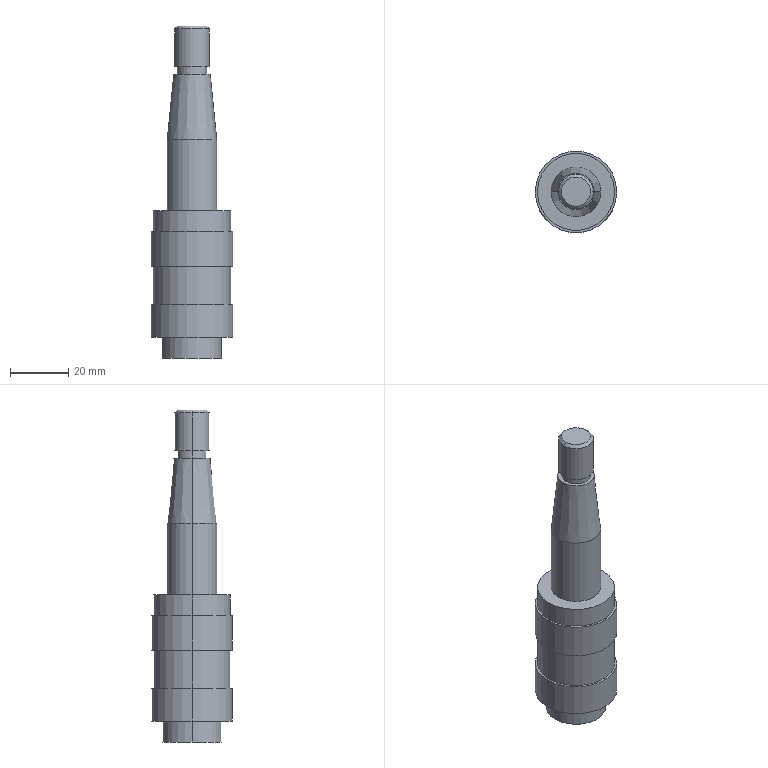Part | SolidWorks | features BaseBody 1 | 1 solid | 29 faces | box 28 x 28 x 114 mm | volume 38900 mm3 | cylinder 16 | plane 9 | cone 4 | commonest cylinder face diameters 26.5 x4 28 x4 10 x2 12 x2 17 x2 20.275 x2
STEP:
#1=CARTESIAN_POINT('',(0.5987,-67.08,58.));
#2=VERTEX_POINT('',#1);
#3=CARTESIAN_POINT('',(-16.401,-67.08,58.));
#4=VERTEX_POINT('',#3);
#5=CARTESIAN_POINT('',(-7.901,-67.08,58.));
#6=DIRECTION('',(0.,0.,1.));
#7=DIRECTION('',(1.,0.,0.));
#8=AXIS2_PLACEMENT_3D('',#5,#6,#7);
#9=CIRCLE('',#8,8.5);
#10=EDGE_CURVE('',#2,#4,#9,.T.);
#11=ORIENTED_EDGE('',*,*,#10,.T.);
#12=CARTESIAN_POINT('',(-16.401,-67.08,82.499));
#13=VERTEX_POINT('',#12);
#14=CARTESIAN_POINT('',(-16.401,-67.08,58.));
#15=DIRECTION('',(0.,0.,1.));
#16=VECTOR('',#15,1000.);
#17=LINE('',#14,#16);
#18=EDGE_CURVE('',#4,#13,#17,.T.);
#19=ORIENTED_EDGE('',*,*,#18,.T.);
#20=CARTESIAN_POINT('',(0.5987,-67.08,82.499));
#21=VERTEX_POINT('',#20);
#22=CARTESIAN_POINT('',(-7.901,-67.08,82.499));
#23=DIRECTION('',(0.,0.,-1.));
#24=DIRECTION('',(1.,0.,0.));
#25=AXIS2_PLACEMENT_3D('',#22,#23,#24);
#26=CIRCLE('',#25,8.5);
#27=EDGE_CURVE('',#13,#21,#26,.T.);
#28=ORIENTED_EDGE('',*,*,#27,.T.);
#29=CARTESIAN_POINT('',(0.5987,-67.08,58.));
#30=DIRECTION('',(0.,0.,1.));
#31=VECTOR('',#30,1000.);
#32=LINE('',#29,#31);
#33=EDGE_CURVE('',#2,#21,#32,.T.);
#34=ORIENTED_EDGE('',*,*,#33,.F.);
#35=EDGE_LOOP('',(#11,#19,#28,#34));
#36=FACE_OUTER_BOUND('',#35,.T.);
#37=CARTESIAN_POINT('',(-7.901,-67.08,58.));
#38=DIRECTION('',(0.,0.,1.));
#39=DIRECTION('',(1.,0.,0.));
#40=AXIS2_PLACEMENT_3D('',#37,#38,#39);
#41=CYLINDRICAL_SURFACE('',#40,8.5);
#42=ADVANCED_FACE('',(#36),#41,.T.);
#43=CARTESIAN_POINT('',(-14.151,-67.08,105.));
#44=VERTEX_POINT('',#43);
#45=CARTESIAN_POINT('',(-1.651,-67.08,105.));
#46=VERTEX_POINT('',#45);
#47=CARTESIAN_POINT('',(-7.901,-67.08,105.));
#48=DIRECTION('',(0.,0.,-1.));
#49=DIRECTION('',(-1.,0.,0.));
#50=AXIS2_PLACEMENT_3D('',#47,#48,#49);
#51=CIRCLE('',#50,6.25);
#52=EDGE_CURVE('',#44,#46,#51,.T.);
#53=ORIENTED_EDGE('',*,*,#52,.T.);
#54=CARTESIAN_POINT('',(0.5987,-67.08,82.499));
#55=DIRECTION('',(0.09949,0.,-0.995));
#56=VECTOR('',#55,1000.);
#57=LINE('',#54,#56);
#58=EDGE_CURVE('',#46,#21,#57,.T.);
#59=ORIENTED_EDGE('',*,*,#58,.T.);
#60=ORIENTED_EDGE('',*,*,#27,.F.);
#61=CARTESIAN_POINT('',(-16.401,-67.08,82.499));
#62=DIRECTION('',(-0.09949,0.,-0.995));
#63=VECTOR('',#62,1000.);
#64=LINE('',#61,#63);
#65=EDGE_CURVE('',#44,#13,#64,.T.);
#66=ORIENTED_EDGE('',*,*,#65,.F.);
#67=EDGE_LOOP('',(#53,#59,#60,#66));
#68=FACE_OUTER_BOUND('',#67,.T.);
#69=CARTESIAN_POINT('',(-7.901,-67.08,82.499));
#70=DIRECTION('',(0.,0.,-1.));
#71=DIRECTION('',(-1.,0.,0.));
#72=AXIS2_PLACEMENT_3D('',#69,#70,#71);
#73=CONICAL_SURFACE('',#72,8.5,0.09966);
#74=ADVANCED_FACE('',(#68),#73,.T.);
#75=CARTESIAN_POINT('',(5.349,-67.08,51.));
#76=VERTEX_POINT('',#75);
#77=CARTESIAN_POINT('',(-21.151,-67.08,51.));
#78=VERTEX_POINT('',#77);
#79=CARTESIAN_POINT('',(-7.901,-67.08,51.));
#80=DIRECTION('',(0.,0.,1.));
#81=DIRECTION('',(1.,0.,0.));
#82=AXIS2_PLACEMENT_3D('',#79,#80,#81);
#83=CIRCLE('',#82,13.25);
#84=EDGE_CURVE('',#76,#78,#83,.T.);
#85=ORIENTED_EDGE('',*,*,#84,.T.);
#86=CARTESIAN_POINT('',(-21.151,-67.08,58.));
#87=VERTEX_POINT('',#86);
#88=CARTESIAN_POINT('',(-21.151,-67.08,51.));
#89=DIRECTION('',(0.,0.,1.));
#90=VECTOR('',#89,1000.);
#91=LINE('',#88,#90);
#92=EDGE_CURVE('',#78,#87,#91,.T.);
#93=ORIENTED_EDGE('',*,*,#92,.T.);
#94=CARTESIAN_POINT('',(5.349,-67.08,58.));
#95=VERTEX_POINT('',#94);
#96=CARTESIAN_POINT('',(-7.901,-67.08,58.));
#97=DIRECTION('',(0.,0.,1.));
#98=DIRECTION('',(1.,0.,0.));
#99=AXIS2_PLACEMENT_3D('',#96,#97,#98);
#100=CIRCLE('',#99,13.25);
#101=EDGE_CURVE('',#95,#87,#100,.T.);
#102=ORIENTED_EDGE('',*,*,#101,.F.);
#103=CARTESIAN_POINT('',(5.349,-67.08,51.));
#104=DIRECTION('',(0.,0.,1.));
#105=VECTOR('',#104,1000.);
#106=LINE('',#103,#105);
#107=EDGE_CURVE('',#76,#95,#106,.T.);
#108=ORIENTED_EDGE('',*,*,#107,.F.);
#109=EDGE_LOOP('',(#85,#93,#102,#108));
#110=FACE_OUTER_BOUND('',#109,.T.);
#111=CARTESIAN_POINT('',(-7.901,-67.08,51.));
#112=DIRECTION('',(0.,0.,1.));
#113=DIRECTION('',(1.,0.,0.));
#114=AXIS2_PLACEMENT_3D('',#111,#112,#113);
#115=CYLINDRICAL_SURFACE('',#114,13.25);
#116=ADVANCED_FACE('',(#110),#115,.T.);
#117=CARTESIAN_POINT('',(-12.901,-67.08,105.));
#118=VERTEX_POINT('',#117);
#119=CARTESIAN_POINT('',(-2.901,-67.08,105.));
#120=VERTEX_POINT('',#119);
#121=CARTESIAN_POINT('',(-7.901,-67.08,105.));
#122=DIRECTION('',(0.,0.,-1.));
#123=DIRECTION('',(1.,0.,0.));
#124=AXIS2_PLACEMENT_3D('',#121,#122,#123);
#125=CIRCLE('',#124,5.);
#126=EDGE_CURVE('',#118,#120,#125,.T.);
#127=ORIENTED_EDGE('',*,*,#126,.F.);
#128=CARTESIAN_POINT('',(-12.901,-67.08,107.5));
#129=VERTEX_POINT('',#128);
#130=CARTESIAN_POINT('',(-12.901,-67.08,105.));
#131=DIRECTION('',(0.,0.,1.));
#132=VECTOR('',#131,1000.);
#133=LINE('',#130,#132);
#134=EDGE_CURVE('',#118,#129,#133,.T.);
#135=ORIENTED_EDGE('',*,*,#134,.T.);
#136=CARTESIAN_POINT('',(-2.901,-67.08,107.5));
#137=VERTEX_POINT('',#136);
#138=CARTESIAN_POINT('',(-7.901,-67.08,107.5));
#139=DIRECTION('',(0.,0.,-1.));
#140=DIRECTION('',(1.,0.,0.));
#141=AXIS2_PLACEMENT_3D('',#138,#139,#140);
#142=CIRCLE('',#141,5.);
#143=EDGE_CURVE('',#129,#137,#142,.T.);
#144=ORIENTED_EDGE('',*,*,#143,.T.);
#145=CARTESIAN_POINT('',(-2.901,-67.08,105.));
#146=DIRECTION('',(0.,0.,1.));
#147=VECTOR('',#146,1000.);
#148=LINE('',#145,#147);
#149=EDGE_CURVE('',#120,#137,#148,.T.);
#150=ORIENTED_EDGE('',*,*,#149,.F.);
#151=EDGE_LOOP('',(#127,#135,#144,#150));
#152=FACE_OUTER_BOUND('',#151,.T.);
#153=CARTESIAN_POINT('',(-7.901,-67.08,105.));
#154=DIRECTION('',(0.,0.,1.));
#155=DIRECTION('',(1.,0.,0.));
#156=AXIS2_PLACEMENT_3D('',#153,#154,#155);
#157=CYLINDRICAL_SURFACE('',#156,5.);
#158=ADVANCED_FACE('',(#152),#157,.T.);
#159=CARTESIAN_POINT('',(6.099,-67.08,39.));
#160=VERTEX_POINT('',#159);
#161=CARTESIAN_POINT('',(-21.901,-67.08,39.));
#162=VERTEX_POINT('',#161);
#163=CARTESIAN_POINT('',(-7.901,-67.08,39.));
#164=DIRECTION('',(0.,0.,1.));
#165=DIRECTION('',(1.,0.,0.));
#166=AXIS2_PLACEMENT_3D('',#163,#164,#165);
#167=CIRCLE('',#166,14.);
#168=EDGE_CURVE('',#160,#162,#167,.T.);
#169=ORIENTED_EDGE('',*,*,#168,.T.);
#170=CARTESIAN_POINT('',(-21.901,-67.08,51.));
#171=VERTEX_POINT('',#170);
#172=CARTESIAN_POINT('',(-21.901,-67.08,39.));
#173=DIRECTION('',(0.,0.,1.));
#174=VECTOR('',#173,1000.);
#175=LINE('',#172,#174);
#176=EDGE_CURVE('',#162,#171,#175,.T.);
#177=ORIENTED_EDGE('',*,*,#176,.T.);
#178=CARTESIAN_POINT('',(6.099,-67.08,51.));
#179=VERTEX_POINT('',#178);
#180=CARTESIAN_POINT('',(-7.901,-67.08,51.));
#181=DIRECTION('',(0.,0.,1.));
#182=DIRECTION('',(1.,0.,0.));
#183=AXIS2_PLACEMENT_3D('',#180,#181,#182);
#184=CIRCLE('',#183,14.);
#185=EDGE_CURVE('',#179,#171,#184,.T.);
#186=ORIENTED_EDGE('',*,*,#185,.F.);
#187=CARTESIAN_POINT('',(6.099,-67.08,39.));
#188=DIRECTION('',(0.,0.,1.));
#189=VECTOR('',#188,1000.);
#190=LINE('',#187,#189);
#191=EDGE_CURVE('',#160,#179,#190,.T.);
#192=ORIENTED_EDGE('',*,*,#191,.F.);
#193=EDGE_LOOP('',(#169,#177,#186,#192));
#194=FACE_OUTER_BOUND('',#193,.T.);
#195=CARTESIAN_POINT('',(-7.901,-67.08,39.));
#196=DIRECTION('',(0.,0.,1.));
#197=DIRECTION('',(1.,0.,0.));
#198=AXIS2_PLACEMENT_3D('',#195,#196,#197);
#199=CYLINDRICAL_SURFACE('',#198,14.);
#200=ADVANCED_FACE('',(#194),#199,.T.);
#201=CARTESIAN_POINT('',(-1.901,-67.08,107.5));
#202=VERTEX_POINT('',#201);
#203=CARTESIAN_POINT('',(-13.901,-67.08,107.5));
#204=VERTEX_POINT('',#203);
#205=CARTESIAN_POINT('',(-7.901,-67.08,107.5));
#206=DIRECTION('',(0.,0.,1.));
#207=DIRECTION('',(1.,0.,0.));
#208=AXIS2_PLACEMENT_3D('',#205,#206,#207);
#209=CIRCLE('',#208,6.);
#210=EDGE_CURVE('',#202,#204,#209,.T.);
#211=ORIENTED_EDGE('',*,*,#210,.T.);
#212=CARTESIAN_POINT('',(-13.901,-67.08,120.5));
#213=VERTEX_POINT('',#212);
#214=CARTESIAN_POINT('',(-13.901,-67.08,107.5));
#215=DIRECTION('',(0.,0.,1.));
#216=VECTOR('',#215,1000.);
#217=LINE('',#214,#216);
#218=EDGE_CURVE('',#204,#213,#217,.T.);
#219=ORIENTED_EDGE('',*,*,#218,.T.);
#220=CARTESIAN_POINT('',(-1.901,-67.08,120.5));
#221=VERTEX_POINT('',#220);
#222=CARTESIAN_POINT('',(-7.901,-67.08,120.5));
#223=DIRECTION('',(0.,0.,-1.));
#224=DIRECTION('',(1.,0.,0.));
#225=AXIS2_PLACEMENT_3D('',#222,#223,#224);
#226=CIRCLE('',#225,6.);
#227=EDGE_CURVE('',#213,#221,#226,.T.);
#228=ORIENTED_EDGE('',*,*,#227,.T.);
#229=CARTESIAN_POINT('',(-1.901,-67.08,107.5));
#230=DIRECTION('',(0.,0.,1.));
#231=VECTOR('',#230,1000.);
#232=LINE('',#229,#231);
#233=EDGE_CURVE('',#202,#221,#232,.T.);
#234=ORIENTED_EDGE('',*,*,#233,.F.);
#235=EDGE_LOOP('',(#211,#219,#228,#234));
#236=FACE_OUTER_BOUND('',#235,.T.);
#237=CARTESIAN_POINT('',(-7.901,-67.08,107.5));
#238=DIRECTION('',(0.,0.,1.));
#239=DIRECTION('',(1.,0.,0.));
#240=AXIS2_PLACEMENT_3D('',#237,#238,#239);
#241=CYLINDRICAL_SURFACE('',#240,6.);
#242=ADVANCED_FACE('',(#236),#241,.T.);
#243=CARTESIAN_POINT('',(5.349,-67.08,26.));
#244=VERTEX_POINT('',#243);
#245=CARTESIAN_POINT('',(-21.151,-67.08,26.));
#246=VERTEX_POINT('',#245);
#247=CARTESIAN_POINT('',(-7.901,-67.08,26.));
#248=DIRECTION('',(0.,0.,1.));
#249=DIRECTION('',(1.,0.,0.));
#250=AXIS2_PLACEMENT_3D('',#247,#248,#249);
#251=CIRCLE('',#250,13.25);
#252=EDGE_CURVE('',#244,#246,#251,.T.);
#253=ORIENTED_EDGE('',*,*,#252,.T.);
#254=CARTESIAN_POINT('',(-21.151,-67.08,39.));
#255=VERTEX_POINT('',#254);
#256=CARTESIAN_POINT('',(-21.151,-67.08,26.));
#257=DIRECTION('',(0.,0.,1.));
#258=VECTOR('',#257,1000.);
#259=LINE('',#256,#258);
#260=EDGE_CURVE('',#246,#255,#259,.T.);
#261=ORIENTED_EDGE('',*,*,#260,.T.);
#262=CARTESIAN_POINT('',(5.349,-67.08,39.));
#263=VERTEX_POINT('',#262);
#264=CARTESIAN_POINT('',(-7.901,-67.08,39.));
#265=DIRECTION('',(0.,0.,-1.));
#266=DIRECTION('',(1.,0.,0.));
#267=AXIS2_PLACEMENT_3D('',#264,#265,#266);
#268=CIRCLE('',#267,13.25);
#269=EDGE_CURVE('',#255,#263,#268,.T.);
#270=ORIENTED_EDGE('',*,*,#269,.T.);
#271=CARTESIAN_POINT('',(5.349,-67.08,26.));
#272=DIRECTION('',(0.,0.,1.));
#273=VECTOR('',#272,1000.);
#274=LINE('',#271,#273);
#275=EDGE_CURVE('',#244,#263,#274,.T.);
#276=ORIENTED_EDGE('',*,*,#275,.F.);
#277=EDGE_LOOP('',(#253,#261,#270,#276));
#278=FACE_OUTER_BOUND('',#277,.T.);
#279=CARTESIAN_POINT('',(-7.901,-67.08,26.));
#280=DIRECTION('',(0.,0.,1.));
#281=DIRECTION('',(1.,0.,0.));
#282=AXIS2_PLACEMENT_3D('',#279,#280,#281);
#283=CYLINDRICAL_SURFACE('',#282,13.25);
#284=ADVANCED_FACE('',(#278),#283,.T.);
#285=CARTESIAN_POINT('',(-12.901,-67.08,121.5));
#286=VERTEX_POINT('',#285);
#287=CARTESIAN_POINT('',(-2.901,-67.08,121.5));
#288=VERTEX_POINT('',#287);
#289=CARTESIAN_POINT('',(-7.901,-67.08,121.5));
#290=DIRECTION('',(0.,0.,-1.));
#291=DIRECTION('',(-1.,0.,0.));
#292=AXIS2_PLACEMENT_3D('',#289,#290,#291);
#293=CIRCLE('',#292,5.);
#294=EDGE_CURVE('',#286,#288,#293,.T.);
#295=ORIENTED_EDGE('',*,*,#294,.T.);
#296=CARTESIAN_POINT('',(-1.901,-67.08,120.5));
#297=DIRECTION('',(0.7071,0.,-0.7071));
#298=VECTOR('',#297,1000.);
#299=LINE('',#296,#298);
#300=EDGE_CURVE('',#288,#221,#299,.T.);
#301=ORIENTED_EDGE('',*,*,#300,.T.);
#302=ORIENTED_EDGE('',*,*,#227,.F.);
#303=CARTESIAN_POINT('',(-13.901,-67.08,120.5));
#304=DIRECTION('',(-0.7071,0.,-0.7071));
#305=VECTOR('',#304,1000.);
#306=LINE('',#303,#305);
#307=EDGE_CURVE('',#286,#213,#306,.T.);
#308=ORIENTED_EDGE('',*,*,#307,.F.);
#309=EDGE_LOOP('',(#295,#301,#302,#308));
#310=FACE_OUTER_BOUND('',#309,.T.);
#311=CARTESIAN_POINT('',(-7.901,-67.08,120.5));
#312=DIRECTION('',(0.,0.,-1.));
#313=DIRECTION('',(-1.,0.,0.));
#314=AXIS2_PLACEMENT_3D('',#311,#312,#313);
#315=CONICAL_SURFACE('',#314,6.,0.7854);
#316=ADVANCED_FACE('',(#310),#315,.T.);
#317=CARTESIAN_POINT('',(6.099,-67.08,14.7));
#318=VERTEX_POINT('',#317);
#319=CARTESIAN_POINT('',(-21.901,-67.08,14.7));
#320=VERTEX_POINT('',#319);
#321=CARTESIAN_POINT('',(-7.901,-67.08,14.7));
#322=DIRECTION('',(0.,0.,1.));
#323=DIRECTION('',(1.,0.,0.));
#324=AXIS2_PLACEMENT_3D('',#321,#322,#323);
#325=CIRCLE('',#324,14.);
#326=EDGE_CURVE('',#318,#320,#325,.T.);
#327=ORIENTED_EDGE('',*,*,#326,.T.);
#328=CARTESIAN_POINT('',(-21.901,-67.08,26.));
#329=VERTEX_POINT('',#328);
#330=CARTESIAN_POINT('',(-21.901,-67.08,14.7));
#331=DIRECTION('',(0.,0.,1.));
#332=VECTOR('',#331,1000.);
#333=LINE('',#330,#332);
#334=EDGE_CURVE('',#320,#329,#333,.T.);
#335=ORIENTED_EDGE('',*,*,#334,.T.);
#336=CARTESIAN_POINT('',(6.099,-67.08,26.));
#337=VERTEX_POINT('',#336);
#338=CARTESIAN_POINT('',(-7.901,-67.08,26.));
#339=DIRECTION('',(0.,0.,1.));
#340=DIRECTION('',(1.,0.,0.));
#341=AXIS2_PLACEMENT_3D('',#338,#339,#340);
#342=CIRCLE('',#341,14.);
#343=EDGE_CURVE('',#337,#329,#342,.T.);
#344=ORIENTED_EDGE('',*,*,#343,.F.);
#345=CARTESIAN_POINT('',(6.099,-67.08,14.7));
#346=DIRECTION('',(0.,0.,1.));
#347=VECTOR('',#346,1000.);
#348=LINE('',#345,#347);
#349=EDGE_CURVE('',#318,#337,#348,.T.);
#350=ORIENTED_EDGE('',*,*,#349,.F.);
#351=EDGE_LOOP('',(#327,#335,#344,#350));
#352=FACE_OUTER_BOUND('',#351,.T.);
#353=CARTESIAN_POINT('',(-7.901,-67.08,14.7));
#354=DIRECTION('',(0.,0.,1.));
#355=DIRECTION('',(1.,0.,0.));
#356=AXIS2_PLACEMENT_3D('',#353,#354,#355);
#357=CYLINDRICAL_SURFACE('',#356,14.);
#358=ADVANCED_FACE('',(#352),#357,.T.);
#359=CARTESIAN_POINT('',(2.236,-67.08,7.5));
#360=VERTEX_POINT('',#359);
#361=CARTESIAN_POINT('',(-18.039,-67.08,7.5));
#362=VERTEX_POINT('',#361);
#363=CARTESIAN_POINT('',(-7.901,-67.08,7.5));
#364=DIRECTION('',(0.,0.,1.));
#365=DIRECTION('',(1.,0.,0.));
#366=AXIS2_PLACEMENT_3D('',#363,#364,#365);
#367=CIRCLE('',#366,10.137);
#368=EDGE_CURVE('',#360,#362,#367,.T.);
#369=ORIENTED_EDGE('',*,*,#368,.T.);
#370=CARTESIAN_POINT('',(-18.039,-67.08,14.7));
#371=VERTEX_POINT('',#370);
#372=CARTESIAN_POINT('',(-18.039,-67.08,7.5));
#373=DIRECTION('',(0.,0.,1.));
#374=VECTOR('',#373,1000.);
#375=LINE('',#372,#374);
#376=EDGE_CURVE('',#362,#371,#375,.T.);
#377=ORIENTED_EDGE('',*,*,#376,.T.);
#378=CARTESIAN_POINT('',(2.236,-67.08,14.7));
#379=VERTEX_POINT('',#378);
#380=CARTESIAN_POINT('',(-7.901,-67.08,14.7));
#381=DIRECTION('',(0.,0.,-1.));
#382=DIRECTION('',(1.,0.,0.));
#383=AXIS2_PLACEMENT_3D('',#380,#381,#382);
#384=CIRCLE('',#383,10.137);
#385=EDGE_CURVE('',#371,#379,#384,.T.);
#386=ORIENTED_EDGE('',*,*,#385,.T.);
#387=CARTESIAN_POINT('',(2.236,-67.08,7.5));
#388=DIRECTION('',(0.,0.,1.));
#389=VECTOR('',#388,1000.);
#390=LINE('',#387,#389);
#391=EDGE_CURVE('',#360,#379,#390,.T.);
#392=ORIENTED_EDGE('',*,*,#391,.F.);
#393=EDGE_LOOP('',(#369,#377,#386,#392));
#394=FACE_OUTER_BOUND('',#393,.T.);
#395=CARTESIAN_POINT('',(-7.901,-67.08,7.5));
#396=DIRECTION('',(0.,0.,1.));
#397=DIRECTION('',(1.,0.,0.));
#398=AXIS2_PLACEMENT_3D('',#395,#396,#397);
#399=CYLINDRICAL_SURFACE('',#398,10.137);
#400=ADVANCED_FACE('',(#394),#399,.T.);
#401=ORIENTED_EDGE('',*,*,#18,.F.);
#402=CARTESIAN_POINT('',(-7.901,-67.08,58.));
#403=DIRECTION('',(0.,0.,1.));
#404=DIRECTION('',(1.,0.,0.));
#405=AXIS2_PLACEMENT_3D('',#402,#403,#404);
#406=CIRCLE('',#405,8.5);
#407=EDGE_CURVE('',#4,#2,#406,.T.);
#408=ORIENTED_EDGE('',*,*,#407,.T.);
#409=ORIENTED_EDGE('',*,*,#33,.T.);
#410=CARTESIAN_POINT('',(-7.901,-67.08,82.499));
#411=DIRECTION('',(0.,0.,-1.));
#412=DIRECTION('',(1.,0.,0.));
#413=AXIS2_PLACEMENT_3D('',#410,#411,#412);
#414=CIRCLE('',#413,8.5);
#415=EDGE_CURVE('',#21,#13,#414,.T.);
#416=ORIENTED_EDGE('',*,*,#415,.T.);
#417=EDGE_LOOP('',(#401,#408,#409,#416));
#418=FACE_OUTER_BOUND('',#417,.T.);
#419=CARTESIAN_POINT('',(-7.901,-67.08,58.));
#420=DIRECTION('',(0.,0.,1.));
#421=DIRECTION('',(1.,0.,0.));
#422=AXIS2_PLACEMENT_3D('',#419,#420,#421);
#423=CYLINDRICAL_SURFACE('',#422,8.5);
#424=ADVANCED_FACE('',(#418),#423,.T.);
#425=ORIENTED_EDGE('',*,*,#10,.F.);
#426=ORIENTED_EDGE('',*,*,#407,.F.);
#427=EDGE_LOOP('',(#425,#426));
#428=FACE_BOUND('',#427,.T.);
#429=ORIENTED_EDGE('',*,*,#101,.T.);
#430=CARTESIAN_POINT('',(-7.901,-67.08,58.));
#431=DIRECTION('',(0.,0.,1.));
#432=DIRECTION('',(1.,0.,0.));
#433=AXIS2_PLACEMENT_3D('',#430,#431,#432);
#434=CIRCLE('',#433,13.25);
#435=EDGE_CURVE('',#87,#95,#434,.T.);
#436=ORIENTED_EDGE('',*,*,#435,.T.);
#437=EDGE_LOOP('',(#429,#436));
#438=FACE_OUTER_BOUND('',#437,.T.);
#439=CARTESIAN_POINT('',(-7.901,-67.08,58.));
#440=DIRECTION('',(0.,0.,1.));
#441=DIRECTION('',(1.,0.,0.));
#442=AXIS2_PLACEMENT_3D('',#439,#440,#441);
#443=PLANE('',#442);
#444=ADVANCED_FACE('',(#428,#438),#443,.T.);
#445=ORIENTED_EDGE('',*,*,#58,.F.);
#446=CARTESIAN_POINT('',(-7.901,-67.08,105.));
#447=DIRECTION('',(0.,0.,-1.));
#448=DIRECTION('',(-1.,0.,0.));
#449=AXIS2_PLACEMENT_3D('',#446,#447,#448);
#450=CIRCLE('',#449,6.25);
#451=EDGE_CURVE('',#46,#44,#450,.T.);
#452=ORIENTED_EDGE('',*,*,#451,.T.);
#453=ORIENTED_EDGE('',*,*,#65,.T.);
#454=ORIENTED_EDGE('',*,*,#415,.F.);
#455=EDGE_LOOP('',(#445,#452,#453,#454));
#456=FACE_OUTER_BOUND('',#455,.T.);
#457=CARTESIAN_POINT('',(-7.901,-67.08,82.499));
#458=DIRECTION('',(0.,0.,-1.));
#459=DIRECTION('',(-1.,0.,0.));
#460=AXIS2_PLACEMENT_3D('',#457,#458,#459);
#461=CONICAL_SURFACE('',#460,8.5,0.09966);
#462=ADVANCED_FACE('',(#456),#461,.T.);
#463=ORIENTED_EDGE('',*,*,#92,.F.);
#464=CARTESIAN_POINT('',(-7.901,-67.08,51.));
#465=DIRECTION('',(0.,0.,1.));
#466=DIRECTION('',(1.,0.,0.));
#467=AXIS2_PLACEMENT_3D('',#464,#465,#466);
#468=CIRCLE('',#467,13.25);
#469=EDGE_CURVE('',#78,#76,#468,.T.);
#470=ORIENTED_EDGE('',*,*,#469,.T.);
#471=ORIENTED_EDGE('',*,*,#107,.T.);
#472=ORIENTED_EDGE('',*,*,#435,.F.);
#473=EDGE_LOOP('',(#463,#470,#471,#472));
#474=FACE_OUTER_BOUND('',#473,.T.);
#475=CARTESIAN_POINT('',(-7.901,-67.08,51.));
#476=DIRECTION('',(0.,0.,1.));
#477=DIRECTION('',(1.,0.,0.));
#478=AXIS2_PLACEMENT_3D('',#475,#476,#477);
#479=CYLINDRICAL_SURFACE('',#478,13.25);
#480=ADVANCED_FACE('',(#474),#479,.T.);
#481=CARTESIAN_POINT('',(-7.901,-67.08,105.));
#482=DIRECTION('',(0.,0.,-1.));
#483=DIRECTION('',(1.,0.,0.));
#484=AXIS2_PLACEMENT_3D('',#481,#482,#483);
#485=CIRCLE('',#484,5.);
#486=EDGE_CURVE('',#120,#118,#485,.T.);
#487=ORIENTED_EDGE('',*,*,#486,.T.);
#488=ORIENTED_EDGE('',*,*,#126,.T.);
#489=EDGE_LOOP('',(#487,#488));
#490=FACE_BOUND('',#489,.T.);
#491=ORIENTED_EDGE('',*,*,#52,.F.);
#492=ORIENTED_EDGE('',*,*,#451,.F.);
#493=EDGE_LOOP('',(#491,#492));
#494=FACE_OUTER_BOUND('',#493,.T.);
#495=CARTESIAN_POINT('',(-7.901,-67.08,105.));
#496=DIRECTION('',(0.,0.,1.));
#497=DIRECTION('',(1.,0.,0.));
#498=AXIS2_PLACEMENT_3D('',#495,#496,#497);
#499=PLANE('',#498);
#500=ADVANCED_FACE('',(#490,#494),#499,.T.);
#501=ORIENTED_EDGE('',*,*,#84,.F.);
#502=ORIENTED_EDGE('',*,*,#469,.F.);
#503=EDGE_LOOP('',(#501,#502));
#504=FACE_BOUND('',#503,.T.);
#505=ORIENTED_EDGE('',*,*,#185,.T.);
#506=CARTESIAN_POINT('',(-7.901,-67.08,51.));
#507=DIRECTION('',(0.,0.,1.));
#508=DIRECTION('',(1.,0.,0.));
#509=AXIS2_PLACEMENT_3D('',#506,#507,#508);
#510=CIRCLE('',#509,14.);
#511=EDGE_CURVE('',#171,#179,#510,.T.);
#512=ORIENTED_EDGE('',*,*,#511,.T.);
#513=EDGE_LOOP('',(#505,#512));
#514=FACE_OUTER_BOUND('',#513,.T.);
#515=CARTESIAN_POINT('',(-7.901,-67.08,51.));
#516=DIRECTION('',(0.,0.,1.));
#517=DIRECTION('',(1.,0.,0.));
#518=AXIS2_PLACEMENT_3D('',#515,#516,#517);
#519=PLANE('',#518);
#520=ADVANCED_FACE('',(#504,#514),#519,.T.);
#521=ORIENTED_EDGE('',*,*,#134,.F.);
#522=ORIENTED_EDGE('',*,*,#486,.F.);
#523=ORIENTED_EDGE('',*,*,#149,.T.);
#524=CARTESIAN_POINT('',(-7.901,-67.08,107.5));
#525=DIRECTION('',(0.,0.,-1.));
#526=DIRECTION('',(1.,0.,0.));
#527=AXIS2_PLACEMENT_3D('',#524,#525,#526);
#528=CIRCLE('',#527,5.);
#529=EDGE_CURVE('',#137,#129,#528,.T.);
#530=ORIENTED_EDGE('',*,*,#529,.T.);
#531=EDGE_LOOP('',(#521,#522,#523,#530));
#532=FACE_OUTER_BOUND('',#531,.T.);
#533=CARTESIAN_POINT('',(-7.901,-67.08,105.));
#534=DIRECTION('',(0.,0.,1.));
#535=DIRECTION('',(1.,0.,0.));
#536=AXIS2_PLACEMENT_3D('',#533,#534,#535);
#537=CYLINDRICAL_SURFACE('',#536,5.);
#538=ADVANCED_FACE('',(#532),#537,.T.);
#539=ORIENTED_EDGE('',*,*,#176,.F.);
#540=CARTESIAN_POINT('',(-7.901,-67.08,39.));
#541=DIRECTION('',(0.,0.,1.));
#542=DIRECTION('',(1.,0.,0.));
#543=AXIS2_PLACEMENT_3D('',#540,#541,#542);
#544=CIRCLE('',#543,14.);
#545=EDGE_CURVE('',#162,#160,#544,.T.);
#546=ORIENTED_EDGE('',*,*,#545,.T.);
#547=ORIENTED_EDGE('',*,*,#191,.T.);
#548=ORIENTED_EDGE('',*,*,#511,.F.);
#549=EDGE_LOOP('',(#539,#546,#547,#548));
#550=FACE_OUTER_BOUND('',#549,.T.);
#551=CARTESIAN_POINT('',(-7.901,-67.08,39.));
#552=DIRECTION('',(0.,0.,1.));
#553=DIRECTION('',(1.,0.,0.));
#554=AXIS2_PLACEMENT_3D('',#551,#552,#553);
#555=CYLINDRICAL_SURFACE('',#554,14.);
#556=ADVANCED_FACE('',(#550),#555,.T.);
#557=ORIENTED_EDGE('',*,*,#529,.F.);
#558=ORIENTED_EDGE('',*,*,#143,.F.);
#559=EDGE_LOOP('',(#557,#558));
#560=FACE_BOUND('',#559,.T.);
#561=ORIENTED_EDGE('',*,*,#210,.F.);
#562=CARTESIAN_POINT('',(-7.901,-67.08,107.5));
#563=DIRECTION('',(0.,0.,1.));
#564=DIRECTION('',(1.,0.,0.));
#565=AXIS2_PLACEMENT_3D('',#562,#563,#564);
#566=CIRCLE('',#565,6.);
#567=EDGE_CURVE('',#204,#202,#566,.T.);
#568=ORIENTED_EDGE('',*,*,#567,.F.);
#569=EDGE_LOOP('',(#561,#568));
#570=FACE_OUTER_BOUND('',#569,.T.);
#571=CARTESIAN_POINT('',(-7.901,-67.08,107.5));
#572=DIRECTION('',(0.,0.,1.));
#573=DIRECTION('',(1.,0.,0.));
#574=AXIS2_PLACEMENT_3D('',#571,#572,#573);
#575=PLANE('',#574);
#576=ADVANCED_FACE('',(#560,#570),#575,.F.);
#577=CARTESIAN_POINT('',(-7.901,-67.08,39.));
#578=DIRECTION('',(0.,0.,-1.));
#579=DIRECTION('',(1.,0.,0.));
#580=AXIS2_PLACEMENT_3D('',#577,#578,#579);
#581=CIRCLE('',#580,13.25);
#582=EDGE_CURVE('',#263,#255,#581,.T.);
#583=ORIENTED_EDGE('',*,*,#582,.F.);
#584=ORIENTED_EDGE('',*,*,#269,.F.);
#585=EDGE_LOOP('',(#583,#584));
#586=FACE_BOUND('',#585,.T.);
#587=ORIENTED_EDGE('',*,*,#168,.F.);
#588=ORIENTED_EDGE('',*,*,#545,.F.);
#589=EDGE_LOOP('',(#587,#588));
#590=FACE_OUTER_BOUND('',#589,.T.);
#591=CARTESIAN_POINT('',(-7.901,-67.08,39.));
#592=DIRECTION('',(0.,0.,1.));
#593=DIRECTION('',(1.,0.,0.));
#594=AXIS2_PLACEMENT_3D('',#591,#592,#593);
#595=PLANE('',#594);
#596=ADVANCED_FACE('',(#586,#590),#595,.F.);
#597=ORIENTED_EDGE('',*,*,#218,.F.);
#598=ORIENTED_EDGE('',*,*,#567,.T.);
#599=ORIENTED_EDGE('',*,*,#233,.T.);
#600=CARTESIAN_POINT('',(-7.901,-67.08,120.5));
#601=DIRECTION('',(0.,0.,-1.));
#602=DIRECTION('',(1.,0.,0.));
#603=AXIS2_PLACEMENT_3D('',#600,#601,#602);
#604=CIRCLE('',#603,6.);
#605=EDGE_CURVE('',#221,#213,#604,.T.);
#606=ORIENTED_EDGE('',*,*,#605,.T.);
#607=EDGE_LOOP('',(#597,#598,#599,#606));
#608=FACE_OUTER_BOUND('',#607,.T.);
#609=CARTESIAN_POINT('',(-7.901,-67.08,107.5));
#610=DIRECTION('',(0.,0.,1.));
#611=DIRECTION('',(1.,0.,0.));
#612=AXIS2_PLACEMENT_3D('',#609,#610,#611);
#613=CYLINDRICAL_SURFACE('',#612,6.);
#614=ADVANCED_FACE('',(#608),#613,.T.);
#615=ORIENTED_EDGE('',*,*,#260,.F.);
#616=CARTESIAN_POINT('',(-7.901,-67.08,26.));
#617=DIRECTION('',(0.,0.,1.));
#618=DIRECTION('',(1.,0.,0.));
#619=AXIS2_PLACEMENT_3D('',#616,#617,#618);
#620=CIRCLE('',#619,13.25);
#621=EDGE_CURVE('',#246,#244,#620,.T.);
#622=ORIENTED_EDGE('',*,*,#621,.T.);
#623=ORIENTED_EDGE('',*,*,#275,.T.);
#624=ORIENTED_EDGE('',*,*,#582,.T.);
#625=EDGE_LOOP('',(#615,#622,#623,#624));
#626=FACE_OUTER_BOUND('',#625,.T.);
#627=CARTESIAN_POINT('',(-7.901,-67.08,26.));
#628=DIRECTION('',(0.,0.,1.));
#629=DIRECTION('',(1.,0.,0.));
#630=AXIS2_PLACEMENT_3D('',#627,#628,#629);
#631=CYLINDRICAL_SURFACE('',#630,13.25);
#632=ADVANCED_FACE('',(#626),#631,.T.);
#633=ORIENTED_EDGE('',*,*,#300,.F.);
#634=CARTESIAN_POINT('',(-7.901,-67.08,121.5));
#635=DIRECTION('',(0.,0.,-1.));
#636=DIRECTION('',(-1.,0.,0.));
#637=AXIS2_PLACEMENT_3D('',#634,#635,#636);
#638=CIRCLE('',#637,5.);
#639=EDGE_CURVE('',#288,#286,#638,.T.);
#640=ORIENTED_EDGE('',*,*,#639,.T.);
#641=ORIENTED_EDGE('',*,*,#307,.T.);
#642=ORIENTED_EDGE('',*,*,#605,.F.);
#643=EDGE_LOOP('',(#633,#640,#641,#642));
#644=FACE_OUTER_BOUND('',#643,.T.);
#645=CARTESIAN_POINT('',(-7.901,-67.08,120.5));
#646=DIRECTION('',(0.,0.,-1.));
#647=DIRECTION('',(-1.,0.,0.));
#648=AXIS2_PLACEMENT_3D('',#645,#646,#647);
#649=CONICAL_SURFACE('',#648,6.,0.7854);
#650=ADVANCED_FACE('',(#644),#649,.T.);
#651=ORIENTED_EDGE('',*,*,#252,.F.);
#652=ORIENTED_EDGE('',*,*,#621,.F.);
#653=EDGE_LOOP('',(#651,#652));
#654=FACE_BOUND('',#653,.T.);
#655=ORIENTED_EDGE('',*,*,#343,.T.);
#656=CARTESIAN_POINT('',(-7.901,-67.08,26.));
#657=DIRECTION('',(0.,0.,1.));
#658=DIRECTION('',(1.,0.,0.));
#659=AXIS2_PLACEMENT_3D('',#656,#657,#658);
#660=CIRCLE('',#659,14.);
#661=EDGE_CURVE('',#329,#337,#660,.T.);
#662=ORIENTED_EDGE('',*,*,#661,.T.);
#663=EDGE_LOOP('',(#655,#662));
#664=FACE_OUTER_BOUND('',#663,.T.);
#665=CARTESIAN_POINT('',(-7.901,-67.08,26.));
#666=DIRECTION('',(0.,0.,1.));
#667=DIRECTION('',(1.,0.,0.));
#668=AXIS2_PLACEMENT_3D('',#665,#666,#667);
#669=PLANE('',#668);
#670=ADVANCED_FACE('',(#654,#664),#669,.T.);
#671=ORIENTED_EDGE('',*,*,#294,.F.);
#672=ORIENTED_EDGE('',*,*,#639,.F.);
#673=EDGE_LOOP('',(#671,#672));
#674=FACE_OUTER_BOUND('',#673,.T.);
#675=CARTESIAN_POINT('',(-7.901,-67.08,121.5));
#676=DIRECTION('',(0.,0.,1.));
#677=DIRECTION('',(1.,0.,0.));
#678=AXIS2_PLACEMENT_3D('',#675,#676,#677);
#679=PLANE('',#678);
#680=ADVANCED_FACE('',(#674),#679,.T.);
#681=ORIENTED_EDGE('',*,*,#334,.F.);
#682=CARTESIAN_POINT('',(-7.901,-67.08,14.7));
#683=DIRECTION('',(0.,0.,1.));
#684=DIRECTION('',(1.,0.,0.));
#685=AXIS2_PLACEMENT_3D('',#682,#683,#684);
#686=CIRCLE('',#685,14.);
#687=EDGE_CURVE('',#320,#318,#686,.T.);
#688=ORIENTED_EDGE('',*,*,#687,.T.);
#689=ORIENTED_EDGE('',*,*,#349,.T.);
#690=ORIENTED_EDGE('',*,*,#661,.F.);
#691=EDGE_LOOP('',(#681,#688,#689,#690));
#692=FACE_OUTER_BOUND('',#691,.T.);
#693=CARTESIAN_POINT('',(-7.901,-67.08,14.7));
#694=DIRECTION('',(0.,0.,1.));
#695=DIRECTION('',(1.,0.,0.));
#696=AXIS2_PLACEMENT_3D('',#693,#694,#695);
#697=CYLINDRICAL_SURFACE('',#696,14.);
#698=ADVANCED_FACE('',(#692),#697,.T.);
#699=CARTESIAN_POINT('',(-7.901,-67.08,14.7));
#700=DIRECTION('',(0.,0.,-1.));
#701=DIRECTION('',(1.,0.,0.));
#702=AXIS2_PLACEMENT_3D('',#699,#700,#701);
#703=CIRCLE('',#702,10.137);
#704=EDGE_CURVE('',#379,#371,#703,.T.);
#705=ORIENTED_EDGE('',*,*,#704,.F.);
#706=ORIENTED_EDGE('',*,*,#385,.F.);
#707=EDGE_LOOP('',(#705,#706));
#708=FACE_BOUND('',#707,.T.);
#709=ORIENTED_EDGE('',*,*,#326,.F.);
#710=ORIENTED_EDGE('',*,*,#687,.F.);
#711=EDGE_LOOP('',(#709,#710));
#712=FACE_OUTER_BOUND('',#711,.T.);
#713=CARTESIAN_POINT('',(-7.901,-67.08,14.7));
#714=DIRECTION('',(0.,0.,1.));
#715=DIRECTION('',(1.,0.,0.));
#716=AXIS2_PLACEMENT_3D('',#713,#714,#715);
#717=PLANE('',#716);
#718=ADVANCED_FACE('',(#708,#712),#717,.F.);
#719=ORIENTED_EDGE('',*,*,#376,.F.);
#720=CARTESIAN_POINT('',(-7.901,-67.08,7.5));
#721=DIRECTION('',(0.,0.,1.));
#722=DIRECTION('',(1.,0.,0.));
#723=AXIS2_PLACEMENT_3D('',#720,#721,#722);
#724=CIRCLE('',#723,10.137);
#725=EDGE_CURVE('',#362,#360,#724,.T.);
#726=ORIENTED_EDGE('',*,*,#725,.T.);
#727=ORIENTED_EDGE('',*,*,#391,.T.);
#728=ORIENTED_EDGE('',*,*,#704,.T.);
#729=EDGE_LOOP('',(#719,#726,#727,#728));
#730=FACE_OUTER_BOUND('',#729,.T.);
#731=CARTESIAN_POINT('',(-7.901,-67.08,7.5));
#732=DIRECTION('',(0.,0.,1.));
#733=DIRECTION('',(1.,0.,0.));
#734=AXIS2_PLACEMENT_3D('',#731,#732,#733);
#735=CYLINDRICAL_SURFACE('',#734,10.137);
#736=ADVANCED_FACE('',(#730),#735,.T.);
#737=ORIENTED_EDGE('',*,*,#368,.F.);
#738=ORIENTED_EDGE('',*,*,#725,.F.);
#739=EDGE_LOOP('',(#737,#738));
#740=FACE_OUTER_BOUND('',#739,.T.);
#741=CARTESIAN_POINT('',(-7.901,-67.08,7.5));
#742=DIRECTION('',(0.,0.,1.));
#743=DIRECTION('',(1.,0.,0.));
#744=AXIS2_PLACEMENT_3D('',#741,#742,#743);
#745=PLANE('',#744);
#746=ADVANCED_FACE('',(#740),#745,.F.);
#747=CLOSED_SHELL('',(#42,#74,#116,#158,#200,#242,#284,#316,#358,#400,#424,#444,#462,#480,#500,#520,#538,#556,#576,#596,#614,#632,#650,#670,#680,#698,#718,#736,#746));
#748=MANIFOLD_SOLID_BREP('',#747);
#749=CARTESIAN_POINT('',(0.,0.,0.));
#750=DIRECTION('',(0.,0.,1.));
#751=DIRECTION('',(1.,0.,0.));
#752=AXIS2_PLACEMENT_3D('',#749,#750,#751);
#753=(LENGTH_UNIT()NAMED_UNIT(*)SI_UNIT(.MILLI.,.METRE.));
#754=UNCERTAINTY_MEASURE_WITH_UNIT(LENGTH_MEASURE(0.00001),#753,'','');
#755=(NAMED_UNIT(*)PLANE_ANGLE_UNIT()SI_UNIT($,.RADIAN.));
#756=(NAMED_UNIT(*)SI_UNIT($,.STERADIAN.)SOLID_ANGLE_UNIT());
#757=(GEOMETRIC_REPRESENTATION_CONTEXT(3)GLOBAL_UNCERTAINTY_ASSIGNED_CONTEXT((#754))GLOBAL_UNIT_ASSIGNED_CONTEXT((#753,#755,#756))REPRESENTATION_CONTEXT('',''));
#758=ADVANCED_BREP_SHAPE_REPRESENTATION('',(#748,#752),#757);